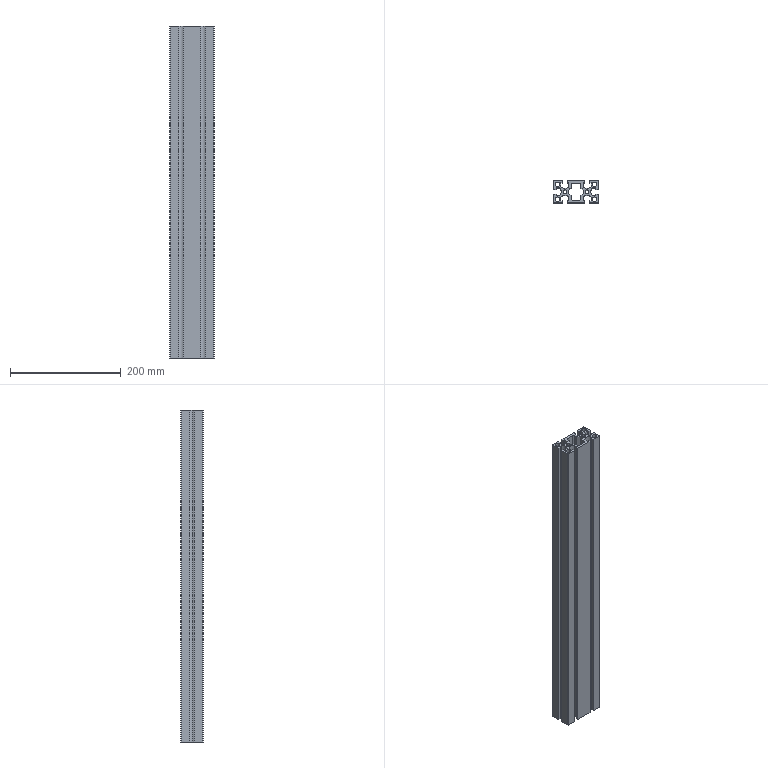Part | STEP file | 40x80 aluminium profile (L=600) | 1 solid | 87 faces | box 80 x 40 x 600 mm | volume 800472 mm3 | plane 60 | cylinder 27 | commonest cylinder face diameters 8 x8 17.549 x7 1 x4 4 x4 6.8 x4